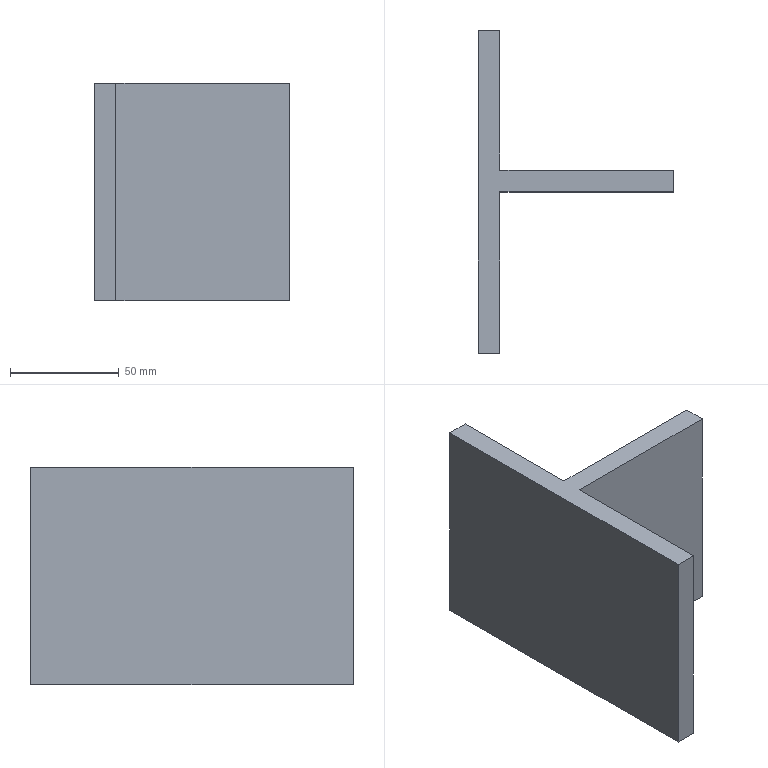Part | STEP file | Mirror slide plate 2 | 1 solid | 10 faces | box 90 x 148.62 x 100 mm | volume 228620 mm3 | plane 10
STEP:
#1=CARTESIAN_POINT('',(40.,0.,-50.));
#2=VERTEX_POINT('',#1);
#3=CARTESIAN_POINT('',(40.,0.,50.));
#4=VERTEX_POINT('',#3);
#5=CARTESIAN_POINT('',(40.,0.,50.));
#6=DIRECTION('',(0.,0.,1.));
#7=VECTOR('',#6,1000.);
#8=LINE('',#5,#7);
#9=EDGE_CURVE('',#2,#4,#8,.T.);
#10=ORIENTED_EDGE('',*,*,#9,.F.);
#11=CARTESIAN_POINT('',(40.,10.,-50.));
#12=VERTEX_POINT('',#11);
#13=CARTESIAN_POINT('',(40.,10.,-50.));
#14=DIRECTION('',(0.,-1.,0.));
#15=VECTOR('',#14,1000.);
#16=LINE('',#13,#15);
#17=EDGE_CURVE('',#12,#2,#16,.T.);
#18=ORIENTED_EDGE('',*,*,#17,.F.);
#19=CARTESIAN_POINT('',(40.,10.,50.));
#20=VERTEX_POINT('',#19);
#21=CARTESIAN_POINT('',(40.,10.,50.));
#22=DIRECTION('',(0.,0.,1.));
#23=VECTOR('',#22,1000.);
#24=LINE('',#21,#23);
#25=EDGE_CURVE('',#12,#20,#24,.T.);
#26=ORIENTED_EDGE('',*,*,#25,.T.);
#27=CARTESIAN_POINT('',(40.,10.,50.));
#28=DIRECTION('',(0.,-1.,0.));
#29=VECTOR('',#28,1000.);
#30=LINE('',#27,#29);
#31=EDGE_CURVE('',#20,#4,#30,.T.);
#32=ORIENTED_EDGE('',*,*,#31,.T.);
#33=EDGE_LOOP('',(#10,#18,#26,#32));
#34=FACE_OUTER_BOUND('',#33,.T.);
#35=CARTESIAN_POINT('',(40.,10.,50.));
#36=DIRECTION('',(-1.,0.,0.));
#37=DIRECTION('',(0.,0.,-1.));
#38=AXIS2_PLACEMENT_3D('',#35,#36,#37);
#39=PLANE('',#38);
#40=ADVANCED_FACE('',(#34),#39,.F.);
#41=CARTESIAN_POINT('',(-40.,0.,50.));
#42=VERTEX_POINT('',#41);
#43=CARTESIAN_POINT('',(-40.,0.,50.));
#44=DIRECTION('',(-1.,0.,0.));
#45=VECTOR('',#44,1000.);
#46=LINE('',#43,#45);
#47=EDGE_CURVE('',#4,#42,#46,.T.);
#48=ORIENTED_EDGE('',*,*,#47,.F.);
#49=ORIENTED_EDGE('',*,*,#31,.F.);
#50=CARTESIAN_POINT('',(-40.,10.,50.));
#51=VERTEX_POINT('',#50);
#52=CARTESIAN_POINT('',(-40.,10.,50.));
#53=DIRECTION('',(-1.,0.,0.));
#54=VECTOR('',#53,1000.);
#55=LINE('',#52,#54);
#56=EDGE_CURVE('',#20,#51,#55,.T.);
#57=ORIENTED_EDGE('',*,*,#56,.T.);
#58=CARTESIAN_POINT('',(-40.,74.31,50.));
#59=VERTEX_POINT('',#58);
#60=CARTESIAN_POINT('',(-40.,74.31,50.));
#61=DIRECTION('',(0.,-1.,0.));
#62=VECTOR('',#61,1000.);
#63=LINE('',#60,#62);
#64=EDGE_CURVE('',#59,#51,#63,.T.);
#65=ORIENTED_EDGE('',*,*,#64,.F.);
#66=CARTESIAN_POINT('',(-50.,74.31,50.));
#67=VERTEX_POINT('',#66);
#68=CARTESIAN_POINT('',(-50.,74.31,50.));
#69=DIRECTION('',(1.,0.,0.));
#70=VECTOR('',#69,1000.);
#71=LINE('',#68,#70);
#72=EDGE_CURVE('',#67,#59,#71,.T.);
#73=ORIENTED_EDGE('',*,*,#72,.F.);
#74=CARTESIAN_POINT('',(-50.,-74.31,50.));
#75=VERTEX_POINT('',#74);
#76=CARTESIAN_POINT('',(-50.,74.31,50.));
#77=DIRECTION('',(0.,-1.,0.));
#78=VECTOR('',#77,1000.);
#79=LINE('',#76,#78);
#80=EDGE_CURVE('',#67,#75,#79,.T.);
#81=ORIENTED_EDGE('',*,*,#80,.T.);
#82=CARTESIAN_POINT('',(-40.,-74.31,50.));
#83=VERTEX_POINT('',#82);
#84=CARTESIAN_POINT('',(-50.,-74.31,50.));
#85=DIRECTION('',(1.,0.,0.));
#86=VECTOR('',#85,1000.);
#87=LINE('',#84,#86);
#88=EDGE_CURVE('',#75,#83,#87,.T.);
#89=ORIENTED_EDGE('',*,*,#88,.T.);
#90=CARTESIAN_POINT('',(-40.,74.31,50.));
#91=DIRECTION('',(0.,-1.,0.));
#92=VECTOR('',#91,1000.);
#93=LINE('',#90,#92);
#94=EDGE_CURVE('',#42,#83,#93,.T.);
#95=ORIENTED_EDGE('',*,*,#94,.F.);
#96=EDGE_LOOP('',(#48,#49,#57,#65,#73,#81,#89,#95));
#97=FACE_OUTER_BOUND('',#96,.T.);
#98=CARTESIAN_POINT('',(-40.,10.,50.));
#99=DIRECTION('',(0.,0.,-1.));
#100=DIRECTION('',(1.,0.,0.));
#101=AXIS2_PLACEMENT_3D('',#98,#99,#100);
#102=PLANE('',#101);
#103=ADVANCED_FACE('',(#97),#102,.F.);
#104=CARTESIAN_POINT('',(-40.,0.,-50.));
#105=VERTEX_POINT('',#104);
#106=CARTESIAN_POINT('',(-40.,0.,-50.));
#107=DIRECTION('',(1.,0.,0.));
#108=VECTOR('',#107,1000.);
#109=LINE('',#106,#108);
#110=EDGE_CURVE('',#105,#2,#109,.T.);
#111=ORIENTED_EDGE('',*,*,#110,.F.);
#112=CARTESIAN_POINT('',(-40.,-74.31,-50.));
#113=VERTEX_POINT('',#112);
#114=CARTESIAN_POINT('',(-40.,74.31,-50.));
#115=DIRECTION('',(0.,1.,0.));
#116=VECTOR('',#115,1000.);
#117=LINE('',#114,#116);
#118=EDGE_CURVE('',#113,#105,#117,.T.);
#119=ORIENTED_EDGE('',*,*,#118,.F.);
#120=CARTESIAN_POINT('',(-50.,-74.31,-50.));
#121=VERTEX_POINT('',#120);
#122=CARTESIAN_POINT('',(-50.,-74.31,-50.));
#123=DIRECTION('',(1.,0.,0.));
#124=VECTOR('',#123,1000.);
#125=LINE('',#122,#124);
#126=EDGE_CURVE('',#121,#113,#125,.T.);
#127=ORIENTED_EDGE('',*,*,#126,.F.);
#128=CARTESIAN_POINT('',(-50.,74.31,-50.));
#129=VERTEX_POINT('',#128);
#130=CARTESIAN_POINT('',(-50.,74.31,-50.));
#131=DIRECTION('',(0.,1.,0.));
#132=VECTOR('',#131,1000.);
#133=LINE('',#130,#132);
#134=EDGE_CURVE('',#121,#129,#133,.T.);
#135=ORIENTED_EDGE('',*,*,#134,.T.);
#136=CARTESIAN_POINT('',(-40.,74.31,-50.));
#137=VERTEX_POINT('',#136);
#138=CARTESIAN_POINT('',(-50.,74.31,-50.));
#139=DIRECTION('',(1.,0.,0.));
#140=VECTOR('',#139,1000.);
#141=LINE('',#138,#140);
#142=EDGE_CURVE('',#129,#137,#141,.T.);
#143=ORIENTED_EDGE('',*,*,#142,.T.);
#144=CARTESIAN_POINT('',(-40.,10.,-50.));
#145=VERTEX_POINT('',#144);
#146=CARTESIAN_POINT('',(-40.,74.31,-50.));
#147=DIRECTION('',(0.,1.,0.));
#148=VECTOR('',#147,1000.);
#149=LINE('',#146,#148);
#150=EDGE_CURVE('',#145,#137,#149,.T.);
#151=ORIENTED_EDGE('',*,*,#150,.F.);
#152=CARTESIAN_POINT('',(-40.,10.,-50.));
#153=DIRECTION('',(1.,0.,0.));
#154=VECTOR('',#153,1000.);
#155=LINE('',#152,#154);
#156=EDGE_CURVE('',#145,#12,#155,.T.);
#157=ORIENTED_EDGE('',*,*,#156,.T.);
#158=ORIENTED_EDGE('',*,*,#17,.T.);
#159=EDGE_LOOP('',(#111,#119,#127,#135,#143,#151,#157,#158));
#160=FACE_OUTER_BOUND('',#159,.T.);
#161=CARTESIAN_POINT('',(-40.,10.,-50.));
#162=DIRECTION('',(0.,0.,1.));
#163=DIRECTION('',(-1.,0.,0.));
#164=AXIS2_PLACEMENT_3D('',#161,#162,#163);
#165=PLANE('',#164);
#166=ADVANCED_FACE('',(#160),#165,.F.);
#167=ORIENTED_EDGE('',*,*,#25,.F.);
#168=ORIENTED_EDGE('',*,*,#156,.F.);
#169=CARTESIAN_POINT('',(-40.,10.,50.));
#170=DIRECTION('',(0.,0.,-1.));
#171=VECTOR('',#170,1000.);
#172=LINE('',#169,#171);
#173=EDGE_CURVE('',#51,#145,#172,.T.);
#174=ORIENTED_EDGE('',*,*,#173,.F.);
#175=ORIENTED_EDGE('',*,*,#56,.F.);
#176=EDGE_LOOP('',(#167,#168,#174,#175));
#177=FACE_OUTER_BOUND('',#176,.T.);
#178=CARTESIAN_POINT('',(0.,10.,0.));
#179=DIRECTION('',(0.,1.,0.));
#180=DIRECTION('',(0.,0.,-1.));
#181=AXIS2_PLACEMENT_3D('',#178,#179,#180);
#182=PLANE('',#181);
#183=ADVANCED_FACE('',(#177),#182,.T.);
#184=ORIENTED_EDGE('',*,*,#9,.T.);
#185=ORIENTED_EDGE('',*,*,#47,.T.);
#186=CARTESIAN_POINT('',(-40.,0.,50.));
#187=DIRECTION('',(0.,0.,-1.));
#188=VECTOR('',#187,1000.);
#189=LINE('',#186,#188);
#190=EDGE_CURVE('',#42,#105,#189,.T.);
#191=ORIENTED_EDGE('',*,*,#190,.T.);
#192=ORIENTED_EDGE('',*,*,#110,.T.);
#193=EDGE_LOOP('',(#184,#185,#191,#192));
#194=FACE_OUTER_BOUND('',#193,.T.);
#195=CARTESIAN_POINT('',(0.,0.,0.));
#196=DIRECTION('',(0.,1.,0.));
#197=DIRECTION('',(0.,0.,-1.));
#198=AXIS2_PLACEMENT_3D('',#195,#196,#197);
#199=PLANE('',#198);
#200=ADVANCED_FACE('',(#194),#199,.F.);
#201=ORIENTED_EDGE('',*,*,#94,.T.);
#202=CARTESIAN_POINT('',(-40.,-74.31,50.));
#203=DIRECTION('',(0.,0.,-1.));
#204=VECTOR('',#203,1000.);
#205=LINE('',#202,#204);
#206=EDGE_CURVE('',#83,#113,#205,.T.);
#207=ORIENTED_EDGE('',*,*,#206,.T.);
#208=ORIENTED_EDGE('',*,*,#118,.T.);
#209=ORIENTED_EDGE('',*,*,#190,.F.);
#210=EDGE_LOOP('',(#201,#207,#208,#209));
#211=FACE_OUTER_BOUND('',#210,.T.);
#212=CARTESIAN_POINT('',(-40.,0.,0.));
#213=DIRECTION('',(-1.,0.,0.));
#214=DIRECTION('',(0.,0.,-1.));
#215=AXIS2_PLACEMENT_3D('',#212,#213,#214);
#216=PLANE('',#215);
#217=ADVANCED_FACE('',(#211),#216,.F.);
#218=CARTESIAN_POINT('',(-40.,74.31,50.));
#219=DIRECTION('',(0.,0.,1.));
#220=VECTOR('',#219,1000.);
#221=LINE('',#218,#220);
#222=EDGE_CURVE('',#137,#59,#221,.T.);
#223=ORIENTED_EDGE('',*,*,#222,.F.);
#224=ORIENTED_EDGE('',*,*,#142,.F.);
#225=CARTESIAN_POINT('',(-50.,74.31,50.));
#226=DIRECTION('',(0.,0.,1.));
#227=VECTOR('',#226,1000.);
#228=LINE('',#225,#227);
#229=EDGE_CURVE('',#129,#67,#228,.T.);
#230=ORIENTED_EDGE('',*,*,#229,.T.);
#231=ORIENTED_EDGE('',*,*,#72,.T.);
#232=EDGE_LOOP('',(#223,#224,#230,#231));
#233=FACE_OUTER_BOUND('',#232,.T.);
#234=CARTESIAN_POINT('',(-50.,74.31,50.));
#235=DIRECTION('',(0.,-1.,0.));
#236=DIRECTION('',(0.,0.,1.));
#237=AXIS2_PLACEMENT_3D('',#234,#235,#236);
#238=PLANE('',#237);
#239=ADVANCED_FACE('',(#233),#238,.F.);
#240=ORIENTED_EDGE('',*,*,#206,.F.);
#241=ORIENTED_EDGE('',*,*,#88,.F.);
#242=CARTESIAN_POINT('',(-50.,-74.31,50.));
#243=DIRECTION('',(0.,0.,-1.));
#244=VECTOR('',#243,1000.);
#245=LINE('',#242,#244);
#246=EDGE_CURVE('',#75,#121,#245,.T.);
#247=ORIENTED_EDGE('',*,*,#246,.T.);
#248=ORIENTED_EDGE('',*,*,#126,.T.);
#249=EDGE_LOOP('',(#240,#241,#247,#248));
#250=FACE_OUTER_BOUND('',#249,.T.);
#251=CARTESIAN_POINT('',(-50.,-74.31,50.));
#252=DIRECTION('',(0.,1.,0.));
#253=DIRECTION('',(0.,0.,-1.));
#254=AXIS2_PLACEMENT_3D('',#251,#252,#253);
#255=PLANE('',#254);
#256=ADVANCED_FACE('',(#250),#255,.F.);
#257=ORIENTED_EDGE('',*,*,#134,.F.);
#258=ORIENTED_EDGE('',*,*,#246,.F.);
#259=ORIENTED_EDGE('',*,*,#80,.F.);
#260=ORIENTED_EDGE('',*,*,#229,.F.);
#261=EDGE_LOOP('',(#257,#258,#259,#260));
#262=FACE_OUTER_BOUND('',#261,.T.);
#263=CARTESIAN_POINT('',(-50.,0.,0.));
#264=DIRECTION('',(-1.,0.,0.));
#265=DIRECTION('',(0.,0.,-1.));
#266=AXIS2_PLACEMENT_3D('',#263,#264,#265);
#267=PLANE('',#266);
#268=ADVANCED_FACE('',(#262),#267,.T.);
#269=ORIENTED_EDGE('',*,*,#173,.T.);
#270=ORIENTED_EDGE('',*,*,#150,.T.);
#271=ORIENTED_EDGE('',*,*,#222,.T.);
#272=ORIENTED_EDGE('',*,*,#64,.T.);
#273=EDGE_LOOP('',(#269,#270,#271,#272));
#274=FACE_OUTER_BOUND('',#273,.T.);
#275=CARTESIAN_POINT('',(-40.,0.,0.));
#276=DIRECTION('',(-1.,0.,0.));
#277=DIRECTION('',(0.,0.,-1.));
#278=AXIS2_PLACEMENT_3D('',#275,#276,#277);
#279=PLANE('',#278);
#280=ADVANCED_FACE('',(#274),#279,.F.);
#281=CLOSED_SHELL('',(#40,#103,#166,#183,#200,#217,#239,#256,#268,#280));
#282=MANIFOLD_SOLID_BREP('',#281);
#283=CARTESIAN_POINT('',(0.,0.,0.));
#284=DIRECTION('',(0.,0.,1.));
#285=DIRECTION('',(1.,0.,0.));
#286=AXIS2_PLACEMENT_3D('',#283,#284,#285);
#287=(LENGTH_UNIT()NAMED_UNIT(*)SI_UNIT(.MILLI.,.METRE.));
#288=UNCERTAINTY_MEASURE_WITH_UNIT(LENGTH_MEASURE(0.00001),#287,'','');
#289=(NAMED_UNIT(*)PLANE_ANGLE_UNIT()SI_UNIT($,.RADIAN.));
#290=(NAMED_UNIT(*)SI_UNIT($,.STERADIAN.)SOLID_ANGLE_UNIT());
#291=(GEOMETRIC_REPRESENTATION_CONTEXT(3)GLOBAL_UNCERTAINTY_ASSIGNED_CONTEXT((#288))GLOBAL_UNIT_ASSIGNED_CONTEXT((#287,#289,#290))REPRESENTATION_CONTEXT('',''));
#292=ADVANCED_BREP_SHAPE_REPRESENTATION('',(#282,#286),#291);